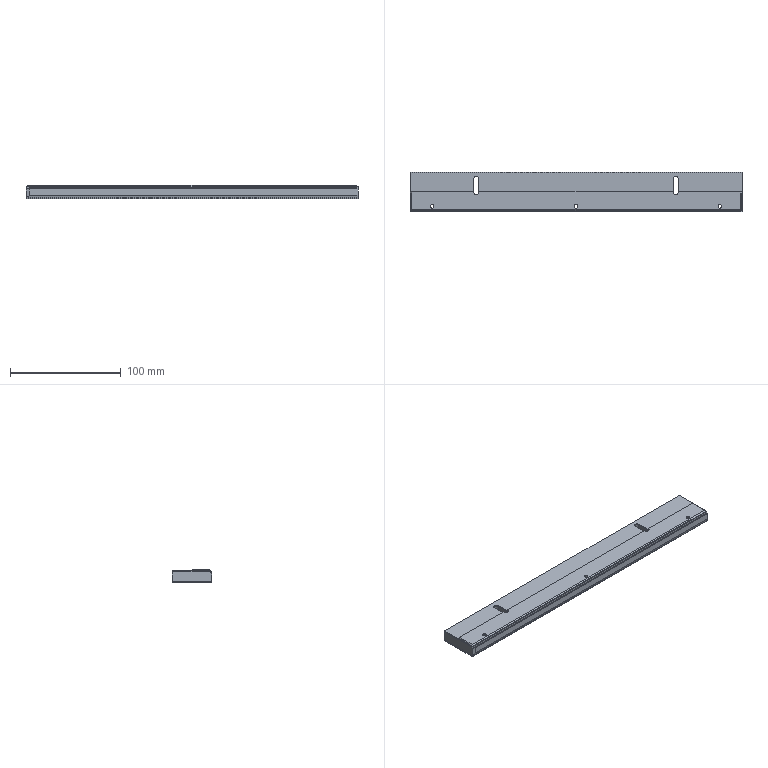Part | 2 solids | 58 faces | box 300 x 36 x 12 mm | volume 219102 mm3 | plane 44 | cylinder 14 | commonest cylinder face diameters 4.5 x8 3.242 x6